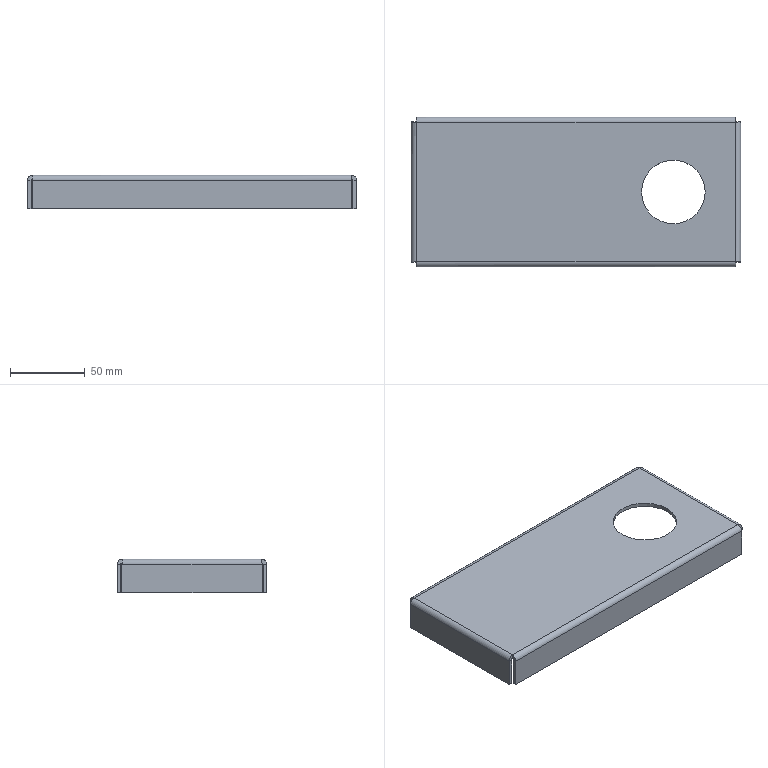Part | SolidWorks | features BaseBody 1 | 1 solid | 40 faces | box 220 x 100 x 22.5 mm | volume 80575 mm3 | plane 22 | cylinder 10 | spline 8 | commonest cylinder face diameters 2 x4 7 x4 42.5 x2